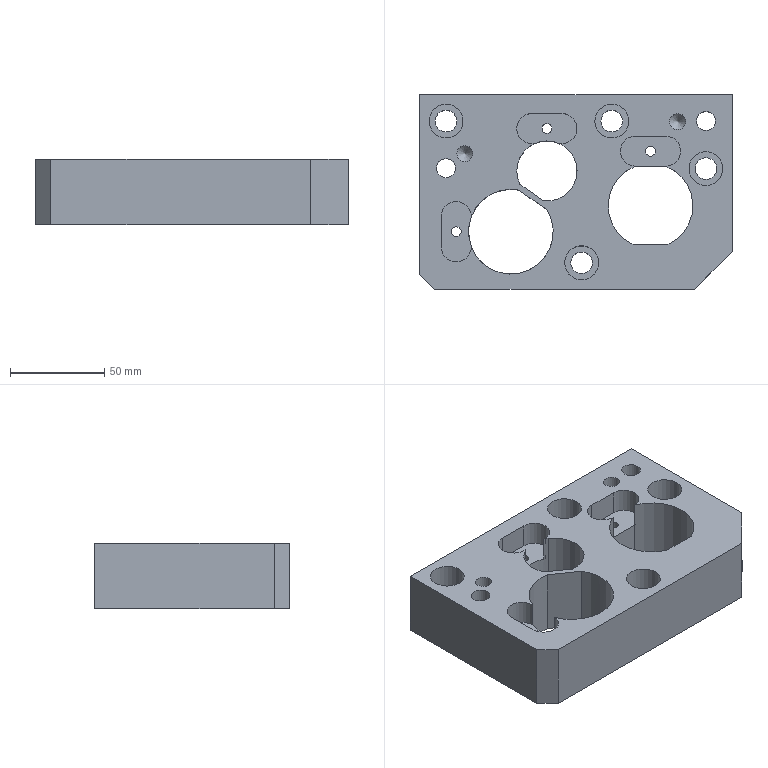Part | STEP file | lll_id4526_x_t | 1 solid | 52 faces | box 166 x 103.25 x 35 mm | volume 405165 mm3 | cylinder 26 | plane 24 | cone 2 | commonest cylinder face diameters 16 x6 11.509 x4 18.008 x4 5.206 x3 45 x3 8.506 x2
STEP:
#1=CARTESIAN_POINT('',(3428.774,36.5,-35.));
#2=VERTEX_POINT('',#1);
#3=CARTESIAN_POINT('',(3427.578,78.,-35.));
#4=VERTEX_POINT('',#3);
#5=CARTESIAN_POINT('',(3419.5,57.,-35.));
#6=DIRECTION('',(0.,0.,1.));
#7=DIRECTION('',(-1.,0.,0.));
#8=AXIS2_PLACEMENT_3D('',#5,#6,#7);
#9=CIRCLE('',#8,22.5);
#10=EDGE_CURVE('',#2,#4,#9,.T.);
#11=ORIENTED_EDGE('',*,*,#10,.F.);
#12=CARTESIAN_POINT('',(3428.774,36.5,0.));
#13=VERTEX_POINT('',#12);
#14=CARTESIAN_POINT('',(3428.774,36.5,0.));
#15=DIRECTION('',(0.,0.,-1.));
#16=VECTOR('',#15,1.);
#17=LINE('',#14,#16);
#18=EDGE_CURVE('',#13,#2,#17,.T.);
#19=ORIENTED_EDGE('',*,*,#18,.F.);
#20=CARTESIAN_POINT('',(3427.578,78.,0.));
#21=VERTEX_POINT('',#20);
#22=CARTESIAN_POINT('',(3419.5,57.,0.));
#23=DIRECTION('',(0.,0.,-1.));
#24=DIRECTION('',(1.,0.,0.));
#25=AXIS2_PLACEMENT_3D('',#22,#23,#24);
#26=CIRCLE('',#25,22.5);
#27=EDGE_CURVE('',#21,#13,#26,.T.);
#28=ORIENTED_EDGE('',*,*,#27,.F.);
#29=CARTESIAN_POINT('',(3427.578,78.,-30.));
#30=DIRECTION('',(0.,0.,-1.));
#31=VECTOR('',#30,1.);
#32=LINE('',#29,#31);
#33=EDGE_CURVE('',#21,#4,#32,.T.);
#34=ORIENTED_EDGE('',*,*,#33,.T.);
#35=EDGE_LOOP('',(#11,#19,#28,#34));
#36=FACE_OUTER_BOUND('',#35,.T.);
#37=CARTESIAN_POINT('',(3419.5,57.,-15.));
#38=DIRECTION('',(0.,0.,-1.));
#39=DIRECTION('',(0.,-1.,0.));
#40=AXIS2_PLACEMENT_3D('',#37,#38,#39);
#41=CYLINDRICAL_SURFACE('',#40,22.5);
#42=ADVANCED_FACE('',(#36),#41,.F.);
#43=CARTESIAN_POINT('',(3411.5,78.,0.));
#44=VERTEX_POINT('',#43);
#45=CARTESIAN_POINT('',(3411.5,78.,-13.));
#46=VERTEX_POINT('',#45);
#47=CARTESIAN_POINT('',(3411.5,78.,-6.5));
#48=DIRECTION('',(0.,0.,-1.));
#49=VECTOR('',#48,1.);
#50=LINE('',#47,#49);
#51=EDGE_CURVE('',#44,#46,#50,.T.);
#52=ORIENTED_EDGE('',*,*,#51,.F.);
#53=CARTESIAN_POINT('',(3411.422,78.,0.));
#54=VERTEX_POINT('',#53);
#55=CARTESIAN_POINT('',(3419.5,78.,0.));
#56=DIRECTION('',(-1.,0.,0.));
#57=VECTOR('',#56,1.);
#58=LINE('',#55,#57);
#59=EDGE_CURVE('',#44,#54,#58,.T.);
#60=ORIENTED_EDGE('',*,*,#59,.T.);
#61=CARTESIAN_POINT('',(3411.422,78.,-35.));
#62=VERTEX_POINT('',#61);
#63=CARTESIAN_POINT('',(3411.422,78.,0.00001771));
#64=DIRECTION('',(0.,0.,1.));
#65=VECTOR('',#64,1.);
#66=LINE('',#63,#65);
#67=EDGE_CURVE('',#62,#54,#66,.T.);
#68=ORIENTED_EDGE('',*,*,#67,.F.);
#69=CARTESIAN_POINT('',(3419.5,78.,-35.));
#70=DIRECTION('',(-1.,0.,0.));
#71=VECTOR('',#70,1.);
#72=LINE('',#69,#71);
#73=EDGE_CURVE('',#4,#62,#72,.T.);
#74=ORIENTED_EDGE('',*,*,#73,.F.);
#75=ORIENTED_EDGE('',*,*,#33,.F.);
#76=CARTESIAN_POINT('',(3427.5,78.,0.));
#77=VERTEX_POINT('',#76);
#78=CARTESIAN_POINT('',(3419.5,78.,0.));
#79=DIRECTION('',(-1.,0.,0.));
#80=VECTOR('',#79,1.);
#81=LINE('',#78,#80);
#82=EDGE_CURVE('',#21,#77,#81,.T.);
#83=ORIENTED_EDGE('',*,*,#82,.T.);
#84=CARTESIAN_POINT('',(3427.5,78.,-13.));
#85=VERTEX_POINT('',#84);
#86=CARTESIAN_POINT('',(3427.5,78.,-6.5));
#87=DIRECTION('',(0.,0.,-1.));
#88=VECTOR('',#87,1.);
#89=LINE('',#86,#88);
#90=EDGE_CURVE('',#77,#85,#89,.T.);
#91=ORIENTED_EDGE('',*,*,#90,.T.);
#92=CARTESIAN_POINT('',(3766.92,78.,-13.));
#93=DIRECTION('',(1.,0.,0.));
#94=VECTOR('',#93,1.);
#95=LINE('',#92,#94);
#96=EDGE_CURVE('',#46,#85,#95,.T.);
#97=ORIENTED_EDGE('',*,*,#96,.F.);
#98=EDGE_LOOP('',(#52,#60,#68,#74,#75,#83,#91,#97));
#99=FACE_OUTER_BOUND('',#98,.T.);
#100=CARTESIAN_POINT('',(3419.5,78.,-32.5));
#101=DIRECTION('',(0.,1.,0.));
#102=DIRECTION('',(0.,0.,-1.));
#103=AXIS2_PLACEMENT_3D('',#100,#101,#102);
#104=PLANE('',#103);
#105=ADVANCED_FACE('',(#99),#104,.F.);
#106=CARTESIAN_POINT('',(3357.736,90.,0.));
#107=VERTEX_POINT('',#106);
#108=CARTESIAN_POINT('',(3357.736,90.,-13.));
#109=VERTEX_POINT('',#108);
#110=CARTESIAN_POINT('',(3357.736,90.,-17.5));
#111=DIRECTION('',(0.,0.,-1.));
#112=VECTOR('',#111,1.);
#113=LINE('',#110,#112);
#114=EDGE_CURVE('',#107,#109,#113,.T.);
#115=ORIENTED_EDGE('',*,*,#114,.F.);
#116=CARTESIAN_POINT('',(3350.125,68.475,0.));
#117=VERTEX_POINT('',#116);
#118=CARTESIAN_POINT('',(3364.5,75.5,0.));
#119=DIRECTION('',(0.,0.,1.));
#120=DIRECTION('',(-1.,0.,0.));
#121=AXIS2_PLACEMENT_3D('',#118,#119,#120);
#122=CIRCLE('',#121,16.);
#123=EDGE_CURVE('',#107,#117,#122,.T.);
#124=ORIENTED_EDGE('',*,*,#123,.T.);
#125=CARTESIAN_POINT('',(3350.125,68.475,-35.));
#126=VERTEX_POINT('',#125);
#127=CARTESIAN_POINT('',(3350.125,68.475,-17.5));
#128=DIRECTION('',(0.,0.,-1.));
#129=VECTOR('',#128,1.);
#130=LINE('',#127,#129);
#131=EDGE_CURVE('',#117,#126,#130,.T.);
#132=ORIENTED_EDGE('',*,*,#131,.T.);
#133=CARTESIAN_POINT('',(3373.677,88.607,-35.));
#134=VERTEX_POINT('',#133);
#135=CARTESIAN_POINT('',(3364.5,75.5,-35.));
#136=DIRECTION('',(0.,0.,-1.));
#137=DIRECTION('',(-1.,0.,0.));
#138=AXIS2_PLACEMENT_3D('',#135,#136,#137);
#139=CIRCLE('',#138,16.);
#140=EDGE_CURVE('',#126,#134,#139,.T.);
#141=ORIENTED_EDGE('',*,*,#140,.T.);
#142=CARTESIAN_POINT('',(3373.677,88.607,0.));
#143=VERTEX_POINT('',#142);
#144=CARTESIAN_POINT('',(3373.677,88.607,-17.5));
#145=DIRECTION('',(0.,0.,-1.));
#146=VECTOR('',#145,1.);
#147=LINE('',#144,#146);
#148=EDGE_CURVE('',#143,#134,#147,.T.);
#149=ORIENTED_EDGE('',*,*,#148,.F.);
#150=CARTESIAN_POINT('',(3371.264,90.,0.));
#151=VERTEX_POINT('',#150);
#152=CARTESIAN_POINT('',(3364.5,75.5,0.));
#153=DIRECTION('',(0.,0.,1.));
#154=DIRECTION('',(-1.,0.,0.));
#155=AXIS2_PLACEMENT_3D('',#152,#153,#154);
#156=CIRCLE('',#155,16.);
#157=EDGE_CURVE('',#143,#151,#156,.T.);
#158=ORIENTED_EDGE('',*,*,#157,.T.);
#159=CARTESIAN_POINT('',(3371.264,90.,-13.));
#160=VERTEX_POINT('',#159);
#161=CARTESIAN_POINT('',(3371.264,90.,-17.5));
#162=DIRECTION('',(0.,0.,1.));
#163=VECTOR('',#162,1.);
#164=LINE('',#161,#163);
#165=EDGE_CURVE('',#160,#151,#164,.T.);
#166=ORIENTED_EDGE('',*,*,#165,.F.);
#167=CARTESIAN_POINT('',(3364.5,75.5,-13.));
#168=DIRECTION('',(0.,0.,-1.));
#169=DIRECTION('',(1.,0.,0.));
#170=AXIS2_PLACEMENT_3D('',#167,#168,#169);
#171=CIRCLE('',#170,16.);
#172=EDGE_CURVE('',#109,#160,#171,.T.);
#173=ORIENTED_EDGE('',*,*,#172,.F.);
#174=EDGE_LOOP('',(#115,#124,#132,#141,#149,#158,#166,#173));
#175=FACE_OUTER_BOUND('',#174,.T.);
#176=CARTESIAN_POINT('',(3364.5,75.5,-17.5));
#177=DIRECTION('',(0.,0.,1.));
#178=DIRECTION('',(-0.5736,-0.8192,0.));
#179=AXIS2_PLACEMENT_3D('',#176,#177,#178);
#180=CYLINDRICAL_SURFACE('',#179,16.);
#181=ADVANCED_FACE('',(#175),#180,.F.);
#182=ORIENTED_EDGE('',*,*,#27,.T.);
#183=CARTESIAN_POINT('',(3410.226,36.5,0.));
#184=VERTEX_POINT('',#183);
#185=CARTESIAN_POINT('',(0.,36.5,0.));
#186=DIRECTION('',(1.,0.,0.));
#187=VECTOR('',#186,1.);
#188=LINE('',#185,#187);
#189=EDGE_CURVE('',#184,#13,#188,.T.);
#190=ORIENTED_EDGE('',*,*,#189,.F.);
#191=CARTESIAN_POINT('',(3419.5,57.,0.));
#192=DIRECTION('',(0.,0.,-1.));
#193=DIRECTION('',(1.,0.,0.));
#194=AXIS2_PLACEMENT_3D('',#191,#192,#193);
#195=CIRCLE('',#194,22.5);
#196=EDGE_CURVE('',#184,#54,#195,.T.);
#197=ORIENTED_EDGE('',*,*,#196,.T.);
#198=ORIENTED_EDGE('',*,*,#59,.F.);
#199=CARTESIAN_POINT('',(3411.5,94.,0.));
#200=VERTEX_POINT('',#199);
#201=CARTESIAN_POINT('',(3411.5,86.,0.));
#202=DIRECTION('',(0.,0.,1.));
#203=DIRECTION('',(0.,-1.,0.));
#204=AXIS2_PLACEMENT_3D('',#201,#202,#203);
#205=CIRCLE('',#204,8.);
#206=EDGE_CURVE('',#200,#44,#205,.T.);
#207=ORIENTED_EDGE('',*,*,#206,.F.);
#208=CARTESIAN_POINT('',(3427.5,94.,0.));
#209=VERTEX_POINT('',#208);
#210=CARTESIAN_POINT('',(3408.538,94.,0.));
#211=DIRECTION('',(1.,0.,0.));
#212=VECTOR('',#211,1.);
#213=LINE('',#210,#212);
#214=EDGE_CURVE('',#200,#209,#213,.T.);
#215=ORIENTED_EDGE('',*,*,#214,.T.);
#216=CARTESIAN_POINT('',(3427.5,86.,0.));
#217=DIRECTION('',(0.,0.,1.));
#218=DIRECTION('',(0.,-1.,0.));
#219=AXIS2_PLACEMENT_3D('',#216,#217,#218);
#220=CIRCLE('',#219,8.);
#221=EDGE_CURVE('',#77,#209,#220,.T.);
#222=ORIENTED_EDGE('',*,*,#221,.F.);
#223=ORIENTED_EDGE('',*,*,#82,.F.);
#224=EDGE_LOOP('',(#182,#190,#197,#198,#207,#215,#222,#223));
#225=FACE_BOUND('',#224,.T.);
#226=CARTESIAN_POINT('',(3308.367,35.288,0.));
#227=VERTEX_POINT('',#226);
#228=CARTESIAN_POINT('',(3324.366,35.211,0.));
#229=VERTEX_POINT('',#228);
#230=CARTESIAN_POINT('',(3316.367,35.288,0.));
#231=DIRECTION('',(0.,0.,1.));
#232=DIRECTION('',(1.,0.,0.));
#233=AXIS2_PLACEMENT_3D('',#230,#231,#232);
#234=CIRCLE('',#233,8.);
#235=EDGE_CURVE('',#227,#229,#234,.T.);
#236=ORIENTED_EDGE('',*,*,#235,.F.);
#237=CARTESIAN_POINT('',(3308.367,51.288,0.));
#238=VERTEX_POINT('',#237);
#239=CARTESIAN_POINT('',(3308.367,32.325,0.));
#240=DIRECTION('',(0.,1.,0.));
#241=VECTOR('',#240,1.);
#242=LINE('',#239,#241);
#243=EDGE_CURVE('',#227,#238,#242,.T.);
#244=ORIENTED_EDGE('',*,*,#243,.T.);
#245=CARTESIAN_POINT('',(3324.366,51.364,0.));
#246=VERTEX_POINT('',#245);
#247=CARTESIAN_POINT('',(3316.367,51.288,0.));
#248=DIRECTION('',(0.,0.,1.));
#249=DIRECTION('',(1.,0.,0.));
#250=AXIS2_PLACEMENT_3D('',#247,#248,#249);
#251=CIRCLE('',#250,8.);
#252=EDGE_CURVE('',#246,#238,#251,.T.);
#253=ORIENTED_EDGE('',*,*,#252,.F.);
#254=CARTESIAN_POINT('',(3349.528,65.399,0.));
#255=VERTEX_POINT('',#254);
#256=CARTESIAN_POINT('',(3345.367,43.288,0.));
#257=DIRECTION('',(0.,0.,1.));
#258=DIRECTION('',(1.,0.,0.));
#259=AXIS2_PLACEMENT_3D('',#256,#257,#258);
#260=CIRCLE('',#259,22.5);
#261=EDGE_CURVE('',#255,#246,#260,.T.);
#262=ORIENTED_EDGE('',*,*,#261,.F.);
#263=CARTESIAN_POINT('',(3364.721,54.761,0.));
#264=VERTEX_POINT('',#263);
#265=CARTESIAN_POINT('',(3357.125,60.08,0.));
#266=DIRECTION('',(-0.8192,0.5736,0.));
#267=VECTOR('',#266,1.);
#268=LINE('',#265,#267);
#269=EDGE_CURVE('',#264,#255,#268,.T.);
#270=ORIENTED_EDGE('',*,*,#269,.F.);
#271=CARTESIAN_POINT('',(3345.367,43.288,0.));
#272=DIRECTION('',(0.,0.,1.));
#273=DIRECTION('',(1.,0.,0.));
#274=AXIS2_PLACEMENT_3D('',#271,#272,#273);
#275=CIRCLE('',#274,22.5);
#276=EDGE_CURVE('',#229,#264,#275,.T.);
#277=ORIENTED_EDGE('',*,*,#276,.F.);
#278=EDGE_LOOP('',(#236,#244,#253,#262,#270,#277));
#279=FACE_BOUND('',#278,.T.);
#280=CARTESIAN_POINT('',(3442.935,12.75,0.));
#281=VERTEX_POINT('',#280);
#282=CARTESIAN_POINT('',(3304.935,12.75,0.));
#283=VERTEX_POINT('',#282);
#284=CARTESIAN_POINT('',(3266.435,12.75,0.));
#285=DIRECTION('',(-1.,0.,0.));
#286=VECTOR('',#285,1.);
#287=LINE('',#284,#286);
#288=EDGE_CURVE('',#281,#283,#287,.T.);
#289=ORIENTED_EDGE('',*,*,#288,.F.);
#290=CARTESIAN_POINT('',(3462.935,32.75,0.));
#291=VERTEX_POINT('',#290);
#292=CARTESIAN_POINT('',(3455.935,25.75,0.));
#293=DIRECTION('',(0.7071,0.7071,0.));
#294=VECTOR('',#293,1.);
#295=LINE('',#292,#294);
#296=EDGE_CURVE('',#281,#291,#295,.T.);
#297=ORIENTED_EDGE('',*,*,#296,.T.);
#298=CARTESIAN_POINT('',(3462.935,116.,0.));
#299=VERTEX_POINT('',#298);
#300=CARTESIAN_POINT('',(3462.935,215.25,0.));
#301=DIRECTION('',(0.,-1.,0.));
#302=VECTOR('',#301,1.);
#303=LINE('',#300,#302);
#304=EDGE_CURVE('',#299,#291,#303,.T.);
#305=ORIENTED_EDGE('',*,*,#304,.F.);
#306=CARTESIAN_POINT('',(3296.935,116.,0.));
#307=VERTEX_POINT('',#306);
#308=CARTESIAN_POINT('',(3266.435,116.,0.));
#309=DIRECTION('',(-1.,0.,0.));
#310=VECTOR('',#309,1.);
#311=LINE('',#308,#310);
#312=EDGE_CURVE('',#299,#307,#311,.T.);
#313=ORIENTED_EDGE('',*,*,#312,.T.);
#314=CARTESIAN_POINT('',(3296.935,20.75,0.));
#315=VERTEX_POINT('',#314);
#316=CARTESIAN_POINT('',(3296.935,215.25,0.));
#317=DIRECTION('',(0.,-1.,0.));
#318=VECTOR('',#317,1.);
#319=LINE('',#316,#318);
#320=EDGE_CURVE('',#307,#315,#319,.T.);
#321=ORIENTED_EDGE('',*,*,#320,.T.);
#322=CARTESIAN_POINT('',(3179.435,138.25,0.));
#323=DIRECTION('',(0.7071,-0.7071,0.));
#324=VECTOR('',#323,1.);
#325=LINE('',#322,#324);
#326=EDGE_CURVE('',#315,#283,#325,.T.);
#327=ORIENTED_EDGE('',*,*,#326,.T.);
#328=EDGE_LOOP('',(#289,#297,#305,#313,#321,#327));
#329=FACE_BOUND('',#328,.T.);
#330=CARTESIAN_POINT('',(3319.939,102.,0.));
#331=VERTEX_POINT('',#330);
#332=CARTESIAN_POINT('',(3310.935,102.,0.));
#333=DIRECTION('',(0.,0.,1.));
#334=DIRECTION('',(1.,0.,0.));
#335=AXIS2_PLACEMENT_3D('',#332,#333,#334);
#336=CIRCLE('',#335,9.004);
#337=EDGE_CURVE('',#331,#331,#336,.T.);
#338=ORIENTED_EDGE('',*,*,#337,.F.);
#339=EDGE_LOOP('',(#338));
#340=FACE_BOUND('',#339,.T.);
#341=CARTESIAN_POINT('',(3315.935,77.,0.));
#342=VERTEX_POINT('',#341);
#343=CARTESIAN_POINT('',(3310.935,77.,0.));
#344=DIRECTION('',(0.,0.,1.));
#345=DIRECTION('',(1.,0.,0.));
#346=AXIS2_PLACEMENT_3D('',#343,#344,#345);
#347=CIRCLE('',#346,5.);
#348=EDGE_CURVE('',#342,#342,#347,.T.);
#349=ORIENTED_EDGE('',*,*,#348,.F.);
#350=EDGE_LOOP('',(#349));
#351=FACE_BOUND('',#350,.T.);
#352=CARTESIAN_POINT('',(3325.188,84.75,0.));
#353=VERTEX_POINT('',#352);
#354=CARTESIAN_POINT('',(3320.935,84.75,0.));
#355=DIRECTION('',(0.,0.,1.));
#356=DIRECTION('',(1.,0.,0.));
#357=AXIS2_PLACEMENT_3D('',#354,#355,#356);
#358=CIRCLE('',#357,4.253);
#359=EDGE_CURVE('',#353,#353,#358,.T.);
#360=ORIENTED_EDGE('',*,*,#359,.F.);
#361=EDGE_LOOP('',(#360));
#362=FACE_BOUND('',#361,.T.);
#363=CARTESIAN_POINT('',(3391.939,26.75,0.));
#364=VERTEX_POINT('',#363);
#365=CARTESIAN_POINT('',(3382.935,26.75,0.));
#366=DIRECTION('',(0.,0.,1.));
#367=DIRECTION('',(1.,0.,0.));
#368=AXIS2_PLACEMENT_3D('',#365,#366,#367);
#369=CIRCLE('',#368,9.004);
#370=EDGE_CURVE('',#364,#364,#369,.T.);
#371=ORIENTED_EDGE('',*,*,#370,.F.);
#372=EDGE_LOOP('',(#371));
#373=FACE_BOUND('',#372,.T.);
#374=CARTESIAN_POINT('',(3457.939,76.75,0.));
#375=VERTEX_POINT('',#374);
#376=CARTESIAN_POINT('',(3448.935,76.75,0.));
#377=DIRECTION('',(0.,0.,1.));
#378=DIRECTION('',(1.,0.,0.));
#379=AXIS2_PLACEMENT_3D('',#376,#377,#378);
#380=CIRCLE('',#379,9.004);
#381=EDGE_CURVE('',#375,#375,#380,.T.);
#382=ORIENTED_EDGE('',*,*,#381,.F.);
#383=EDGE_LOOP('',(#382));
#384=FACE_BOUND('',#383,.T.);
#385=CARTESIAN_POINT('',(3453.935,102.,0.));
#386=VERTEX_POINT('',#385);
#387=CARTESIAN_POINT('',(3448.935,102.,0.));
#388=DIRECTION('',(0.,0.,1.));
#389=DIRECTION('',(1.,0.,0.));
#390=AXIS2_PLACEMENT_3D('',#387,#388,#389);
#391=CIRCLE('',#390,5.);
#392=EDGE_CURVE('',#386,#386,#391,.T.);
#393=ORIENTED_EDGE('',*,*,#392,.F.);
#394=EDGE_LOOP('',(#393));
#395=FACE_BOUND('',#394,.T.);
#396=CARTESIAN_POINT('',(3407.939,102.,0.));
#397=VERTEX_POINT('',#396);
#398=CARTESIAN_POINT('',(3398.935,102.,0.));
#399=DIRECTION('',(0.,0.,1.));
#400=DIRECTION('',(1.,0.,0.));
#401=AXIS2_PLACEMENT_3D('',#398,#399,#400);
#402=CIRCLE('',#401,9.004);
#403=EDGE_CURVE('',#397,#397,#402,.T.);
#404=ORIENTED_EDGE('',*,*,#403,.F.);
#405=EDGE_LOOP('',(#404));
#406=FACE_BOUND('',#405,.T.);
#407=CARTESIAN_POINT('',(3438.188,101.75,0.));
#408=VERTEX_POINT('',#407);
#409=CARTESIAN_POINT('',(3433.935,101.75,0.));
#410=DIRECTION('',(0.,0.,1.));
#411=DIRECTION('',(1.,0.,0.));
#412=AXIS2_PLACEMENT_3D('',#409,#410,#411);
#413=CIRCLE('',#412,4.253);
#414=EDGE_CURVE('',#408,#408,#413,.T.);
#415=ORIENTED_EDGE('',*,*,#414,.F.);
#416=EDGE_LOOP('',(#415));
#417=FACE_BOUND('',#416,.T.);
#418=ORIENTED_EDGE('',*,*,#123,.F.);
#419=CARTESIAN_POINT('',(3356.5,90.,0.));
#420=VERTEX_POINT('',#419);
#421=CARTESIAN_POINT('',(3353.538,90.,0.));
#422=DIRECTION('',(-1.,0.,0.));
#423=VECTOR('',#422,1.);
#424=LINE('',#421,#423);
#425=EDGE_CURVE('',#107,#420,#424,.T.);
#426=ORIENTED_EDGE('',*,*,#425,.T.);
#427=CARTESIAN_POINT('',(3356.5,106.,0.));
#428=VERTEX_POINT('',#427);
#429=CARTESIAN_POINT('',(3356.5,98.,0.));
#430=DIRECTION('',(0.,0.,1.));
#431=DIRECTION('',(0.,-1.,0.));
#432=AXIS2_PLACEMENT_3D('',#429,#430,#431);
#433=CIRCLE('',#432,8.);
#434=EDGE_CURVE('',#428,#420,#433,.T.);
#435=ORIENTED_EDGE('',*,*,#434,.F.);
#436=CARTESIAN_POINT('',(3372.5,106.,0.));
#437=VERTEX_POINT('',#436);
#438=CARTESIAN_POINT('',(3353.538,106.,0.));
#439=DIRECTION('',(1.,0.,0.));
#440=VECTOR('',#439,1.);
#441=LINE('',#438,#440);
#442=EDGE_CURVE('',#428,#437,#441,.T.);
#443=ORIENTED_EDGE('',*,*,#442,.T.);
#444=CARTESIAN_POINT('',(3372.5,90.,0.));
#445=VERTEX_POINT('',#444);
#446=CARTESIAN_POINT('',(3372.5,98.,0.));
#447=DIRECTION('',(0.,0.,1.));
#448=DIRECTION('',(0.,-1.,0.));
#449=AXIS2_PLACEMENT_3D('',#446,#447,#448);
#450=CIRCLE('',#449,8.);
#451=EDGE_CURVE('',#445,#437,#450,.T.);
#452=ORIENTED_EDGE('',*,*,#451,.F.);
#453=CARTESIAN_POINT('',(3353.538,90.,0.));
#454=DIRECTION('',(-1.,0.,0.));
#455=VECTOR('',#454,1.);
#456=LINE('',#453,#455);
#457=EDGE_CURVE('',#445,#151,#456,.T.);
#458=ORIENTED_EDGE('',*,*,#457,.T.);
#459=ORIENTED_EDGE('',*,*,#157,.F.);
#460=CARTESIAN_POINT('',(3362.815,59.589,0.000008705));
#461=VERTEX_POINT('',#460);
#462=CARTESIAN_POINT('',(3364.5,75.5,0.));
#463=DIRECTION('',(0.,0.,1.));
#464=DIRECTION('',(-1.,0.,0.));
#465=AXIS2_PLACEMENT_3D('',#462,#463,#464);
#466=CIRCLE('',#465,16.);
#467=EDGE_CURVE('',#461,#143,#466,.T.);
#468=ORIENTED_EDGE('',*,*,#467,.F.);
#469=CARTESIAN_POINT('',(3225.007,156.084,0.));
#470=DIRECTION('',(0.8192,-0.5736,0.));
#471=VECTOR('',#470,1.);
#472=LINE('',#469,#471);
#473=EDGE_CURVE('',#117,#461,#472,.T.);
#474=ORIENTED_EDGE('',*,*,#473,.F.);
#475=EDGE_LOOP('',(#418,#426,#435,#443,#452,#458,#459,#468,#474));
#476=FACE_BOUND('',#475,.T.);
#477=CARTESIAN_POINT('',(3266.435,215.25,0.));
#478=DIRECTION('',(0.,0.,1.));
#479=DIRECTION('',(-1.,0.,0.));
#480=AXIS2_PLACEMENT_3D('',#477,#478,#479);
#481=PLANE('',#480);
#482=ADVANCED_FACE('',(#225,#279,#329,#340,#351,#362,#373,#384,#395,#406,#417,#476),#481,.T.);
#483=CARTESIAN_POINT('',(3324.366,35.211,-13.));
#484=VERTEX_POINT('',#483);
#485=CARTESIAN_POINT('',(3324.366,51.364,-13.));
#486=VERTEX_POINT('',#485);
#487=CARTESIAN_POINT('',(3345.367,43.288,-13.));
#488=DIRECTION('',(0.,0.,-1.));
#489=DIRECTION('',(1.,0.,0.));
#490=AXIS2_PLACEMENT_3D('',#487,#488,#489);
#491=CIRCLE('',#490,22.5);
#492=EDGE_CURVE('',#484,#486,#491,.T.);
#493=ORIENTED_EDGE('',*,*,#492,.F.);
#494=CARTESIAN_POINT('',(3324.366,35.211,-6.5));
#495=DIRECTION('',(0.,0.,1.));
#496=VECTOR('',#495,1.);
#497=LINE('',#494,#496);
#498=EDGE_CURVE('',#484,#229,#497,.T.);
#499=ORIENTED_EDGE('',*,*,#498,.T.);
#500=ORIENTED_EDGE('',*,*,#276,.T.);
#501=CARTESIAN_POINT('',(3364.721,54.761,-35.));
#502=VERTEX_POINT('',#501);
#503=CARTESIAN_POINT('',(3364.721,54.761,-15.));
#504=DIRECTION('',(0.,0.,-1.));
#505=VECTOR('',#504,1.);
#506=LINE('',#503,#505);
#507=EDGE_CURVE('',#264,#502,#506,.T.);
#508=ORIENTED_EDGE('',*,*,#507,.T.);
#509=CARTESIAN_POINT('',(3349.528,65.399,-35.));
#510=VERTEX_POINT('',#509);
#511=CARTESIAN_POINT('',(3345.367,43.288,-35.));
#512=DIRECTION('',(0.,0.,1.));
#513=DIRECTION('',(-1.,0.,0.));
#514=AXIS2_PLACEMENT_3D('',#511,#512,#513);
#515=CIRCLE('',#514,22.5);
#516=EDGE_CURVE('',#510,#502,#515,.T.);
#517=ORIENTED_EDGE('',*,*,#516,.F.);
#518=CARTESIAN_POINT('',(3349.528,65.399,-15.));
#519=DIRECTION('',(0.,0.,1.));
#520=VECTOR('',#519,1.);
#521=LINE('',#518,#520);
#522=EDGE_CURVE('',#510,#255,#521,.T.);
#523=ORIENTED_EDGE('',*,*,#522,.T.);
#524=ORIENTED_EDGE('',*,*,#261,.T.);
#525=CARTESIAN_POINT('',(3324.366,51.364,-6.5));
#526=DIRECTION('',(0.,0.,-1.));
#527=VECTOR('',#526,1.);
#528=LINE('',#525,#527);
#529=EDGE_CURVE('',#246,#486,#528,.T.);
#530=ORIENTED_EDGE('',*,*,#529,.T.);
#531=EDGE_LOOP('',(#493,#499,#500,#508,#517,#523,#524,#530));
#532=FACE_OUTER_BOUND('',#531,.T.);
#533=CARTESIAN_POINT('',(3345.367,43.288,-15.));
#534=DIRECTION('',(0.,0.,-1.));
#535=DIRECTION('',(0.8192,-0.5736,0.));
#536=AXIS2_PLACEMENT_3D('',#533,#534,#535);
#537=CYLINDRICAL_SURFACE('',#536,22.5);
#538=ADVANCED_FACE('',(#532),#537,.F.);
#539=ORIENTED_EDGE('',*,*,#467,.T.);
#540=ORIENTED_EDGE('',*,*,#148,.T.);
#541=CARTESIAN_POINT('',(3362.815,59.589,-35.));
#542=VERTEX_POINT('',#541);
#543=CARTESIAN_POINT('',(3364.5,75.5,-35.));
#544=DIRECTION('',(0.,0.,-1.));
#545=DIRECTION('',(-1.,0.,0.));
#546=AXIS2_PLACEMENT_3D('',#543,#544,#545);
#547=CIRCLE('',#546,16.);
#548=EDGE_CURVE('',#134,#542,#547,.T.);
#549=ORIENTED_EDGE('',*,*,#548,.T.);
#550=CARTESIAN_POINT('',(3362.815,59.589,-17.5));
#551=DIRECTION('',(0.,0.,1.));
#552=VECTOR('',#551,1.);
#553=LINE('',#550,#552);
#554=EDGE_CURVE('',#542,#461,#553,.T.);
#555=ORIENTED_EDGE('',*,*,#554,.T.);
#556=EDGE_LOOP('',(#539,#540,#549,#555));
#557=FACE_OUTER_BOUND('',#556,.T.);
#558=CARTESIAN_POINT('',(3364.5,75.5,-17.5));
#559=DIRECTION('',(0.,0.,1.));
#560=DIRECTION('',(-0.5736,-0.8192,0.));
#561=AXIS2_PLACEMENT_3D('',#558,#559,#560);
#562=CYLINDRICAL_SURFACE('',#561,16.);
#563=ADVANCED_FACE('',(#557),#562,.F.);
#564=CARTESIAN_POINT('',(3410.226,36.5,-35.));
#565=VERTEX_POINT('',#564);
#566=CARTESIAN_POINT('',(3410.226,36.5,-15.));
#567=DIRECTION('',(0.,0.,1.));
#568=VECTOR('',#567,1.);
#569=LINE('',#566,#568);
#570=EDGE_CURVE('',#565,#184,#569,.T.);
#571=ORIENTED_EDGE('',*,*,#570,.F.);
#572=CARTESIAN_POINT('',(3419.5,57.,-35.));
#573=DIRECTION('',(0.,0.,1.));
#574=DIRECTION('',(-1.,0.,0.));
#575=AXIS2_PLACEMENT_3D('',#572,#573,#574);
#576=CIRCLE('',#575,22.5);
#577=EDGE_CURVE('',#62,#565,#576,.T.);
#578=ORIENTED_EDGE('',*,*,#577,.F.);
#579=ORIENTED_EDGE('',*,*,#67,.T.);
#580=ORIENTED_EDGE('',*,*,#196,.F.);
#581=EDGE_LOOP('',(#571,#578,#579,#580));
#582=FACE_OUTER_BOUND('',#581,.T.);
#583=CARTESIAN_POINT('',(3419.5,57.,-15.));
#584=DIRECTION('',(0.,0.,-1.));
#585=DIRECTION('',(0.,-1.,0.));
#586=AXIS2_PLACEMENT_3D('',#583,#584,#585);
#587=CYLINDRICAL_SURFACE('',#586,22.5);
#588=ADVANCED_FACE('',(#582),#587,.F.);
#589=ORIENTED_EDGE('',*,*,#522,.F.);
#590=CARTESIAN_POINT('',(3357.125,60.08,-35.));
#591=DIRECTION('',(0.8192,-0.5736,0.));
#592=VECTOR('',#591,1.);
#593=LINE('',#590,#592);
#594=EDGE_CURVE('',#510,#502,#593,.T.);
#595=ORIENTED_EDGE('',*,*,#594,.T.);
#596=ORIENTED_EDGE('',*,*,#507,.F.);
#597=ORIENTED_EDGE('',*,*,#269,.T.);
#598=EDGE_LOOP('',(#589,#595,#596,#597));
#599=FACE_OUTER_BOUND('',#598,.T.);
#600=CARTESIAN_POINT('',(3357.125,60.08,-32.5));
#601=DIRECTION('',(0.5736,0.8192,0.));
#602=DIRECTION('',(0.,0.,1.));
#603=AXIS2_PLACEMENT_3D('',#600,#601,#602);
#604=PLANE('',#603);
#605=ADVANCED_FACE('',(#599),#604,.F.);
#606=ORIENTED_EDGE('',*,*,#554,.F.);
#607=CARTESIAN_POINT('',(3225.007,156.084,-35.));
#608=DIRECTION('',(-0.8192,0.5736,0.));
#609=VECTOR('',#608,1.);
#610=LINE('',#607,#609);
#611=EDGE_CURVE('',#542,#126,#610,.T.);
#612=ORIENTED_EDGE('',*,*,#611,.T.);
#613=ORIENTED_EDGE('',*,*,#131,.F.);
#614=ORIENTED_EDGE('',*,*,#473,.T.);
#615=EDGE_LOOP('',(#606,#612,#613,#614));
#616=FACE_OUTER_BOUND('',#615,.T.);
#617=CARTESIAN_POINT('',(3356.47,64.032,-32.5));
#618=DIRECTION('',(-0.5736,-0.8192,0.));
#619=DIRECTION('',(0.,0.,-1.));
#620=AXIS2_PLACEMENT_3D('',#617,#618,#619);
#621=PLANE('',#620);
#622=ADVANCED_FACE('',(#616),#621,.F.);
#623=CARTESIAN_POINT('',(3304.935,12.75,-35.));
#624=VERTEX_POINT('',#623);
#625=CARTESIAN_POINT('',(3442.935,12.75,-35.));
#626=VERTEX_POINT('',#625);
#627=CARTESIAN_POINT('',(3266.435,12.75,-35.));
#628=DIRECTION('',(1.,0.,0.));
#629=VECTOR('',#628,1.);
#630=LINE('',#627,#629);
#631=EDGE_CURVE('',#624,#626,#630,.T.);
#632=ORIENTED_EDGE('',*,*,#631,.T.);
#633=CARTESIAN_POINT('',(3442.935,12.75,-32.));
#634=DIRECTION('',(0.,0.,1.));
#635=VECTOR('',#634,1.);
#636=LINE('',#633,#635);
#637=EDGE_CURVE('',#626,#281,#636,.T.);
#638=ORIENTED_EDGE('',*,*,#637,.T.);
#639=ORIENTED_EDGE('',*,*,#288,.T.);
#640=CARTESIAN_POINT('',(3304.935,12.75,-35.));
#641=DIRECTION('',(0.,0.,-1.));
#642=VECTOR('',#641,1.);
#643=LINE('',#640,#642);
#644=EDGE_CURVE('',#283,#624,#643,.T.);
#645=ORIENTED_EDGE('',*,*,#644,.T.);
#646=EDGE_LOOP('',(#632,#638,#639,#645));
#647=FACE_OUTER_BOUND('',#646,.T.);
#648=CARTESIAN_POINT('',(3266.435,12.75,-32.));
#649=DIRECTION('',(0.,-1.,0.));
#650=DIRECTION('',(0.,0.,1.));
#651=AXIS2_PLACEMENT_3D('',#648,#649,#650);
#652=PLANE('',#651);
#653=ADVANCED_FACE('',(#647),#652,.T.);
#654=ORIENTED_EDGE('',*,*,#304,.T.);
#655=CARTESIAN_POINT('',(3462.935,32.75,-35.));
#656=VERTEX_POINT('',#655);
#657=CARTESIAN_POINT('',(3462.935,32.75,-32.));
#658=DIRECTION('',(0.,0.,-1.));
#659=VECTOR('',#658,1.);
#660=LINE('',#657,#659);
#661=EDGE_CURVE('',#291,#656,#660,.T.);
#662=ORIENTED_EDGE('',*,*,#661,.T.);
#663=CARTESIAN_POINT('',(3462.935,116.,-35.));
#664=VERTEX_POINT('',#663);
#665=CARTESIAN_POINT('',(3462.935,215.25,-35.));
#666=DIRECTION('',(0.,1.,0.));
#667=VECTOR('',#666,1.);
#668=LINE('',#665,#667);
#669=EDGE_CURVE('',#656,#664,#668,.T.);
#670=ORIENTED_EDGE('',*,*,#669,.T.);
#671=CARTESIAN_POINT('',(3462.935,116.,-32.));
#672=DIRECTION('',(0.,0.,1.));
#673=VECTOR('',#672,1.);
#674=LINE('',#671,#673);
#675=EDGE_CURVE('',#664,#299,#674,.T.);
#676=ORIENTED_EDGE('',*,*,#675,.T.);
#677=EDGE_LOOP('',(#654,#662,#670,#676));
#678=FACE_OUTER_BOUND('',#677,.T.);
#679=CARTESIAN_POINT('',(3462.935,215.25,-32.));
#680=DIRECTION('',(1.,0.,0.));
#681=DIRECTION('',(0.,0.,1.));
#682=AXIS2_PLACEMENT_3D('',#679,#680,#681);
#683=PLANE('',#682);
#684=ADVANCED_FACE('',(#678),#683,.T.);
#685=CARTESIAN_POINT('',(3313.764,43.288,-35.));
#686=VERTEX_POINT('',#685);
#687=CARTESIAN_POINT('',(3316.367,43.288,-35.));
#688=DIRECTION('',(0.,0.,-1.));
#689=DIRECTION('',(-1.,0.,0.));
#690=AXIS2_PLACEMENT_3D('',#687,#688,#689);
#691=CIRCLE('',#690,2.603);
#692=EDGE_CURVE('',#686,#686,#691,.T.);
#693=ORIENTED_EDGE('',*,*,#692,.F.);
#694=EDGE_LOOP('',(#693));
#695=FACE_BOUND('',#694,.T.);
#696=CARTESIAN_POINT('',(3419.5,88.603,-35.));
#697=VERTEX_POINT('',#696);
#698=CARTESIAN_POINT('',(3419.5,86.,-35.));
#699=DIRECTION('',(0.,0.,-1.));
#700=DIRECTION('',(0.,1.,0.));
#701=AXIS2_PLACEMENT_3D('',#698,#699,#700);
#702=CIRCLE('',#701,2.603);
#703=EDGE_CURVE('',#697,#697,#702,.T.);
#704=ORIENTED_EDGE('',*,*,#703,.F.);
#705=EDGE_LOOP('',(#704));
#706=FACE_BOUND('',#705,.T.);
#707=CARTESIAN_POINT('',(3364.5,100.603,-35.));
#708=VERTEX_POINT('',#707);
#709=CARTESIAN_POINT('',(3364.5,98.,-35.));
#710=DIRECTION('',(0.,0.,-1.));
#711=DIRECTION('',(0.,1.,0.));
#712=AXIS2_PLACEMENT_3D('',#709,#710,#711);
#713=CIRCLE('',#712,2.603);
#714=EDGE_CURVE('',#708,#708,#713,.T.);
#715=ORIENTED_EDGE('',*,*,#714,.F.);
#716=EDGE_LOOP('',(#715));
#717=FACE_BOUND('',#716,.T.);
#718=ORIENTED_EDGE('',*,*,#516,.T.);
#719=ORIENTED_EDGE('',*,*,#594,.F.);
#720=EDGE_LOOP('',(#718,#719));
#721=FACE_BOUND('',#720,.T.);
#722=ORIENTED_EDGE('',*,*,#10,.T.);
#723=ORIENTED_EDGE('',*,*,#73,.T.);
#724=ORIENTED_EDGE('',*,*,#577,.T.);
#725=CARTESIAN_POINT('',(0.,36.5,-35.));
#726=DIRECTION('',(-1.,0.,0.));
#727=VECTOR('',#726,1.);
#728=LINE('',#725,#727);
#729=EDGE_CURVE('',#2,#565,#728,.T.);
#730=ORIENTED_EDGE('',*,*,#729,.F.);
#731=EDGE_LOOP('',(#722,#723,#724,#730));
#732=FACE_BOUND('',#731,.T.);
#733=ORIENTED_EDGE('',*,*,#611,.F.);
#734=ORIENTED_EDGE('',*,*,#548,.F.);
#735=ORIENTED_EDGE('',*,*,#140,.F.);
#736=EDGE_LOOP('',(#733,#734,#735));
#737=FACE_BOUND('',#736,.T.);
#738=CARTESIAN_POINT('',(3443.181,76.75,-35.));
#739=VERTEX_POINT('',#738);
#740=CARTESIAN_POINT('',(3448.935,76.75,-35.));
#741=DIRECTION('',(0.,0.,-1.));
#742=DIRECTION('',(-1.,0.,0.));
#743=AXIS2_PLACEMENT_3D('',#740,#741,#742);
#744=CIRCLE('',#743,5.755);
#745=EDGE_CURVE('',#739,#739,#744,.T.);
#746=ORIENTED_EDGE('',*,*,#745,.F.);
#747=EDGE_LOOP('',(#746));
#748=FACE_BOUND('',#747,.T.);
#749=CARTESIAN_POINT('',(3393.181,102.,-35.));
#750=VERTEX_POINT('',#749);
#751=CARTESIAN_POINT('',(3398.935,102.,-35.));
#752=DIRECTION('',(0.,0.,-1.));
#753=DIRECTION('',(-1.,0.,0.));
#754=AXIS2_PLACEMENT_3D('',#751,#752,#753);
#755=CIRCLE('',#754,5.755);
#756=EDGE_CURVE('',#750,#750,#755,.T.);
#757=ORIENTED_EDGE('',*,*,#756,.F.);
#758=EDGE_LOOP('',(#757));
#759=FACE_BOUND('',#758,.T.);
#760=CARTESIAN_POINT('',(3443.935,102.,-35.));
#761=VERTEX_POINT('',#760);
#762=CARTESIAN_POINT('',(3448.935,102.,-35.));
#763=DIRECTION('',(0.,0.,-1.));
#764=DIRECTION('',(-1.,0.,0.));
#765=AXIS2_PLACEMENT_3D('',#762,#763,#764);
#766=CIRCLE('',#765,5.);
#767=EDGE_CURVE('',#761,#761,#766,.T.);
#768=ORIENTED_EDGE('',*,*,#767,.F.);
#769=EDGE_LOOP('',(#768));
#770=FACE_BOUND('',#769,.T.);
#771=CARTESIAN_POINT('',(3377.181,26.75,-35.));
#772=VERTEX_POINT('',#771);
#773=CARTESIAN_POINT('',(3382.935,26.75,-35.));
#774=DIRECTION('',(0.,0.,-1.));
#775=DIRECTION('',(-1.,0.,0.));
#776=AXIS2_PLACEMENT_3D('',#773,#774,#775);
#777=CIRCLE('',#776,5.755);
#778=EDGE_CURVE('',#772,#772,#777,.T.);
#779=ORIENTED_EDGE('',*,*,#778,.F.);
#780=EDGE_LOOP('',(#779));
#781=FACE_BOUND('',#780,.T.);
#782=CARTESIAN_POINT('',(3305.935,77.,-35.));
#783=VERTEX_POINT('',#782);
#784=CARTESIAN_POINT('',(3310.935,77.,-35.));
#785=DIRECTION('',(0.,0.,-1.));
#786=DIRECTION('',(-1.,0.,0.));
#787=AXIS2_PLACEMENT_3D('',#784,#785,#786);
#788=CIRCLE('',#787,5.);
#789=EDGE_CURVE('',#783,#783,#788,.T.);
#790=ORIENTED_EDGE('',*,*,#789,.F.);
#791=EDGE_LOOP('',(#790));
#792=FACE_BOUND('',#791,.T.);
#793=CARTESIAN_POINT('',(3305.181,102.,-35.));
#794=VERTEX_POINT('',#793);
#795=CARTESIAN_POINT('',(3310.935,102.,-35.));
#796=DIRECTION('',(0.,0.,-1.));
#797=DIRECTION('',(-1.,0.,0.));
#798=AXIS2_PLACEMENT_3D('',#795,#796,#797);
#799=CIRCLE('',#798,5.755);
#800=EDGE_CURVE('',#794,#794,#799,.T.);
#801=ORIENTED_EDGE('',*,*,#800,.F.);
#802=EDGE_LOOP('',(#801));
#803=FACE_BOUND('',#802,.T.);
#804=ORIENTED_EDGE('',*,*,#669,.F.);
#805=CARTESIAN_POINT('',(3455.935,25.75,-35.));
#806=DIRECTION('',(-0.7071,-0.7071,0.));
#807=VECTOR('',#806,1.);
#808=LINE('',#805,#807);
#809=EDGE_CURVE('',#656,#626,#808,.T.);
#810=ORIENTED_EDGE('',*,*,#809,.T.);
#811=ORIENTED_EDGE('',*,*,#631,.F.);
#812=CARTESIAN_POINT('',(3296.935,20.75,-35.));
#813=VERTEX_POINT('',#812);
#814=CARTESIAN_POINT('',(3179.435,138.25,-35.));
#815=DIRECTION('',(-0.7071,0.7071,0.));
#816=VECTOR('',#815,1.);
#817=LINE('',#814,#816);
#818=EDGE_CURVE('',#624,#813,#817,.T.);
#819=ORIENTED_EDGE('',*,*,#818,.T.);
#820=CARTESIAN_POINT('',(3296.935,116.,-35.));
#821=VERTEX_POINT('',#820);
#822=CARTESIAN_POINT('',(3296.935,215.25,-35.));
#823=DIRECTION('',(0.,-1.,0.));
#824=VECTOR('',#823,1.);
#825=LINE('',#822,#824);
#826=EDGE_CURVE('',#821,#813,#825,.T.);
#827=ORIENTED_EDGE('',*,*,#826,.F.);
#828=CARTESIAN_POINT('',(3266.435,116.,-35.));
#829=DIRECTION('',(-1.,0.,0.));
#830=VECTOR('',#829,1.);
#831=LINE('',#828,#830);
#832=EDGE_CURVE('',#664,#821,#831,.T.);
#833=ORIENTED_EDGE('',*,*,#832,.F.);
#834=EDGE_LOOP('',(#804,#810,#811,#819,#827,#833));
#835=FACE_BOUND('',#834,.T.);
#836=CARTESIAN_POINT('',(3266.435,215.25,-35.));
#837=DIRECTION('',(0.,0.,-1.));
#838=DIRECTION('',(1.,0.,0.));
#839=AXIS2_PLACEMENT_3D('',#836,#837,#838);
#840=PLANE('',#839);
#841=ADVANCED_FACE('',(#695,#706,#717,#721,#732,#737,#748,#759,#770,#781,#792,#803,#835),#840,.T.);
#842=ORIENTED_EDGE('',*,*,#832,.T.);
#843=CARTESIAN_POINT('',(3296.935,116.,-17.5));
#844=DIRECTION('',(0.,0.,-1.));
#845=VECTOR('',#844,1.);
#846=LINE('',#843,#845);
#847=EDGE_CURVE('',#307,#821,#846,.T.);
#848=ORIENTED_EDGE('',*,*,#847,.F.);
#849=ORIENTED_EDGE('',*,*,#312,.F.);
#850=ORIENTED_EDGE('',*,*,#675,.F.);
#851=EDGE_LOOP('',(#842,#848,#849,#850));
#852=FACE_OUTER_BOUND('',#851,.T.);
#853=CARTESIAN_POINT('',(3384.935,116.,-17.5));
#854=DIRECTION('',(0.,-1.,0.));
#855=DIRECTION('',(0.,0.,-1.));
#856=AXIS2_PLACEMENT_3D('',#853,#854,#855);
#857=PLANE('',#856);
#858=ADVANCED_FACE('',(#852),#857,.F.);
#859=ORIENTED_EDGE('',*,*,#826,.T.);
#860=CARTESIAN_POINT('',(3296.935,20.75,0.));
#861=DIRECTION('',(0.,0.,1.));
#862=VECTOR('',#861,1.);
#863=LINE('',#860,#862);
#864=EDGE_CURVE('',#813,#315,#863,.T.);
#865=ORIENTED_EDGE('',*,*,#864,.T.);
#866=ORIENTED_EDGE('',*,*,#320,.F.);
#867=ORIENTED_EDGE('',*,*,#847,.T.);
#868=EDGE_LOOP('',(#859,#865,#866,#867));
#869=FACE_OUTER_BOUND('',#868,.T.);
#870=CARTESIAN_POINT('',(3296.935,62.,-17.5));
#871=DIRECTION('',(1.,0.,0.));
#872=DIRECTION('',(0.,0.,-1.));
#873=AXIS2_PLACEMENT_3D('',#870,#871,#872);
#874=PLANE('',#873);
#875=ADVANCED_FACE('',(#869),#874,.F.);
#876=ORIENTED_EDGE('',*,*,#800,.T.);
#877=EDGE_LOOP('',(#876));
#878=FACE_BOUND('',#877,.T.);
#879=CARTESIAN_POINT('',(3305.181,102.,-13.));
#880=VERTEX_POINT('',#879);
#881=CARTESIAN_POINT('',(3310.935,102.,-13.));
#882=DIRECTION('',(0.,0.,-1.));
#883=DIRECTION('',(-1.,0.,0.));
#884=AXIS2_PLACEMENT_3D('',#881,#882,#883);
#885=CIRCLE('',#884,5.755);
#886=EDGE_CURVE('',#880,#880,#885,.T.);
#887=ORIENTED_EDGE('',*,*,#886,.F.);
#888=EDGE_LOOP('',(#887));
#889=FACE_BOUND('',#888,.T.);
#890=CARTESIAN_POINT('',(3310.935,102.,2.));
#891=DIRECTION('',(0.,0.,-1.));
#892=DIRECTION('',(1.,0.,0.));
#893=AXIS2_PLACEMENT_3D('',#890,#891,#892);
#894=CYLINDRICAL_SURFACE('',#893,5.755);
#895=ADVANCED_FACE('',(#878,#889),#894,.F.);
#896=ORIENTED_EDGE('',*,*,#886,.T.);
#897=EDGE_LOOP('',(#896));
#898=FACE_BOUND('',#897,.T.);
#899=CARTESIAN_POINT('',(3319.939,102.,-13.));
#900=VERTEX_POINT('',#899);
#901=CARTESIAN_POINT('',(3310.935,102.,-13.));
#902=DIRECTION('',(0.,0.,-1.));
#903=DIRECTION('',(1.,0.,0.));
#904=AXIS2_PLACEMENT_3D('',#901,#902,#903);
#905=CIRCLE('',#904,9.004);
#906=EDGE_CURVE('',#900,#900,#905,.T.);
#907=ORIENTED_EDGE('',*,*,#906,.F.);
#908=EDGE_LOOP('',(#907));
#909=FACE_BOUND('',#908,.T.);
#910=CARTESIAN_POINT('',(3310.935,102.,-13.));
#911=DIRECTION('',(0.,0.,-1.));
#912=DIRECTION('',(-1.,0.,0.));
#913=AXIS2_PLACEMENT_3D('',#910,#911,#912);
#914=PLANE('',#913);
#915=ADVANCED_FACE('',(#898,#909),#914,.F.);
#916=ORIENTED_EDGE('',*,*,#337,.T.);
#917=EDGE_LOOP('',(#916));
#918=FACE_BOUND('',#917,.T.);
#919=ORIENTED_EDGE('',*,*,#906,.T.);
#920=EDGE_LOOP('',(#919));
#921=FACE_BOUND('',#920,.T.);
#922=CARTESIAN_POINT('',(3310.935,102.,0.00007723));
#923=DIRECTION('',(0.,0.,-1.));
#924=DIRECTION('',(1.,0.,0.));
#925=AXIS2_PLACEMENT_3D('',#922,#923,#924);
#926=CYLINDRICAL_SURFACE('',#925,9.004);
#927=ADVANCED_FACE('',(#918,#921),#926,.F.);
#928=ORIENTED_EDGE('',*,*,#789,.T.);
#929=EDGE_LOOP('',(#928));
#930=FACE_BOUND('',#929,.T.);
#931=ORIENTED_EDGE('',*,*,#348,.T.);
#932=EDGE_LOOP('',(#931));
#933=FACE_BOUND('',#932,.T.);
#934=CARTESIAN_POINT('',(3310.935,77.,2.));
#935=DIRECTION('',(0.,0.,-1.));
#936=DIRECTION('',(-1.,0.,0.));
#937=AXIS2_PLACEMENT_3D('',#934,#935,#936);
#938=CYLINDRICAL_SURFACE('',#937,5.);
#939=ADVANCED_FACE('',(#930,#933),#938,.F.);
#940=ORIENTED_EDGE('',*,*,#359,.T.);
#941=EDGE_LOOP('',(#940));
#942=FACE_BOUND('',#941,.T.);
#943=CARTESIAN_POINT('',(3325.188,84.75,-28.753));
#944=VERTEX_POINT('',#943);
#945=CARTESIAN_POINT('',(3320.935,84.75,-28.753));
#946=DIRECTION('',(0.,0.,1.));
#947=DIRECTION('',(1.,0.,0.));
#948=AXIS2_PLACEMENT_3D('',#945,#946,#947);
#949=CIRCLE('',#948,4.253);
#950=EDGE_CURVE('',#944,#944,#949,.T.);
#951=ORIENTED_EDGE('',*,*,#950,.F.);
#952=EDGE_LOOP('',(#951));
#953=FACE_BOUND('',#952,.T.);
#954=CARTESIAN_POINT('',(3320.935,84.75,2.));
#955=DIRECTION('',(0.,0.,-1.));
#956=DIRECTION('',(-1.,0.,0.));
#957=AXIS2_PLACEMENT_3D('',#954,#955,#956);
#958=CYLINDRICAL_SURFACE('',#957,4.253);
#959=ADVANCED_FACE('',(#942,#953),#958,.F.);
#960=CARTESIAN_POINT('',(3320.935,84.75,-33.006));
#961=VERTEX_POINT('',#960);
#962=VERTEX_LOOP('',#961);
#963=FACE_BOUND('',#962,.T.);
#964=ORIENTED_EDGE('',*,*,#950,.T.);
#965=EDGE_LOOP('',(#964));
#966=FACE_BOUND('',#965,.T.);
#967=CARTESIAN_POINT('',(3320.935,84.75,-28.753));
#968=DIRECTION('',(0.,0.,1.));
#969=DIRECTION('',(-1.,0.,0.));
#970=AXIS2_PLACEMENT_3D('',#967,#968,#969);
#971=CONICAL_SURFACE('',#970,4.253,45.);
#972=ADVANCED_FACE('',(#963,#966),#971,.F.);
#973=ORIENTED_EDGE('',*,*,#778,.T.);
#974=EDGE_LOOP('',(#973));
#975=FACE_BOUND('',#974,.T.);
#976=CARTESIAN_POINT('',(3377.181,26.75,-13.));
#977=VERTEX_POINT('',#976);
#978=CARTESIAN_POINT('',(3382.935,26.75,-13.));
#979=DIRECTION('',(0.,0.,-1.));
#980=DIRECTION('',(-1.,0.,0.));
#981=AXIS2_PLACEMENT_3D('',#978,#979,#980);
#982=CIRCLE('',#981,5.755);
#983=EDGE_CURVE('',#977,#977,#982,.T.);
#984=ORIENTED_EDGE('',*,*,#983,.F.);
#985=EDGE_LOOP('',(#984));
#986=FACE_BOUND('',#985,.T.);
#987=CARTESIAN_POINT('',(3382.935,26.75,2.));
#988=DIRECTION('',(0.,0.,-1.));
#989=DIRECTION('',(1.,0.,0.));
#990=AXIS2_PLACEMENT_3D('',#987,#988,#989);
#991=CYLINDRICAL_SURFACE('',#990,5.755);
#992=ADVANCED_FACE('',(#975,#986),#991,.F.);
#993=ORIENTED_EDGE('',*,*,#983,.T.);
#994=EDGE_LOOP('',(#993));
#995=FACE_BOUND('',#994,.T.);
#996=CARTESIAN_POINT('',(3391.939,26.75,-13.));
#997=VERTEX_POINT('',#996);
#998=CARTESIAN_POINT('',(3382.935,26.75,-13.));
#999=DIRECTION('',(0.,0.,-1.));
#1000=DIRECTION('',(1.,0.,0.));
#1001=AXIS2_PLACEMENT_3D('',#998,#999,#1000);
#1002=CIRCLE('',#1001,9.004);
#1003=EDGE_CURVE('',#997,#997,#1002,.T.);
#1004=ORIENTED_EDGE('',*,*,#1003,.F.);
#1005=EDGE_LOOP('',(#1004));
#1006=FACE_BOUND('',#1005,.T.);
#1007=CARTESIAN_POINT('',(3382.935,26.75,-13.));
#1008=DIRECTION('',(0.,0.,-1.));
#1009=DIRECTION('',(-1.,0.,0.));
#1010=AXIS2_PLACEMENT_3D('',#1007,#1008,#1009);
#1011=PLANE('',#1010);
#1012=ADVANCED_FACE('',(#995,#1006),#1011,.F.);
#1013=ORIENTED_EDGE('',*,*,#370,.T.);
#1014=EDGE_LOOP('',(#1013));
#1015=FACE_BOUND('',#1014,.T.);
#1016=ORIENTED_EDGE('',*,*,#1003,.T.);
#1017=EDGE_LOOP('',(#1016));
#1018=FACE_BOUND('',#1017,.T.);
#1019=CARTESIAN_POINT('',(3382.935,26.75,0.00007723));
#1020=DIRECTION('',(0.,0.,-1.));
#1021=DIRECTION('',(1.,0.,0.));
#1022=AXIS2_PLACEMENT_3D('',#1019,#1020,#1021);
#1023=CYLINDRICAL_SURFACE('',#1022,9.004);
#1024=ADVANCED_FACE('',(#1015,#1018),#1023,.F.);
#1025=ORIENTED_EDGE('',*,*,#414,.T.);
#1026=EDGE_LOOP('',(#1025));
#1027=FACE_BOUND('',#1026,.T.);
#1028=CARTESIAN_POINT('',(3429.682,101.75,-28.753));
#1029=VERTEX_POINT('',#1028);
#1030=CARTESIAN_POINT('',(3433.935,101.75,-28.753));
#1031=DIRECTION('',(0.,0.,-1.));
#1032=DIRECTION('',(-1.,0.,0.));
#1033=AXIS2_PLACEMENT_3D('',#1030,#1031,#1032);
#1034=CIRCLE('',#1033,4.253);
#1035=EDGE_CURVE('',#1029,#1029,#1034,.T.);
#1036=ORIENTED_EDGE('',*,*,#1035,.T.);
#1037=EDGE_LOOP('',(#1036));
#1038=FACE_BOUND('',#1037,.T.);
#1039=CARTESIAN_POINT('',(3433.935,101.75,2.));
#1040=DIRECTION('',(0.,0.,-1.));
#1041=DIRECTION('',(1.,0.,0.));
#1042=AXIS2_PLACEMENT_3D('',#1039,#1040,#1041);
#1043=CYLINDRICAL_SURFACE('',#1042,4.253);
#1044=ADVANCED_FACE('',(#1027,#1038),#1043,.F.);
#1045=CARTESIAN_POINT('',(3433.935,101.75,-33.006));
#1046=VERTEX_POINT('',#1045);
#1047=VERTEX_LOOP('',#1046);
#1048=FACE_BOUND('',#1047,.T.);
#1049=ORIENTED_EDGE('',*,*,#1035,.F.);
#1050=EDGE_LOOP('',(#1049));
#1051=FACE_BOUND('',#1050,.T.);
#1052=CARTESIAN_POINT('',(3433.935,101.75,-28.753));
#1053=DIRECTION('',(0.,0.,1.));
#1054=DIRECTION('',(1.,0.,0.));
#1055=AXIS2_PLACEMENT_3D('',#1052,#1053,#1054);
#1056=CONICAL_SURFACE('',#1055,4.253,45.);
#1057=ADVANCED_FACE('',(#1048,#1051),#1056,.F.);
#1058=ORIENTED_EDGE('',*,*,#767,.T.);
#1059=EDGE_LOOP('',(#1058));
#1060=FACE_BOUND('',#1059,.T.);
#1061=ORIENTED_EDGE('',*,*,#392,.T.);
#1062=EDGE_LOOP('',(#1061));
#1063=FACE_BOUND('',#1062,.T.);
#1064=CARTESIAN_POINT('',(3448.935,102.,2.));
#1065=DIRECTION('',(0.,0.,-1.));
#1066=DIRECTION('',(1.,0.,0.));
#1067=AXIS2_PLACEMENT_3D('',#1064,#1065,#1066);
#1068=CYLINDRICAL_SURFACE('',#1067,5.);
#1069=ADVANCED_FACE('',(#1060,#1063),#1068,.F.);
#1070=ORIENTED_EDGE('',*,*,#756,.T.);
#1071=EDGE_LOOP('',(#1070));
#1072=FACE_BOUND('',#1071,.T.);
#1073=CARTESIAN_POINT('',(3393.181,102.,-13.));
#1074=VERTEX_POINT('',#1073);
#1075=CARTESIAN_POINT('',(3398.935,102.,-13.));
#1076=DIRECTION('',(0.,0.,-1.));
#1077=DIRECTION('',(-1.,0.,0.));
#1078=AXIS2_PLACEMENT_3D('',#1075,#1076,#1077);
#1079=CIRCLE('',#1078,5.755);
#1080=EDGE_CURVE('',#1074,#1074,#1079,.T.);
#1081=ORIENTED_EDGE('',*,*,#1080,.F.);
#1082=EDGE_LOOP('',(#1081));
#1083=FACE_BOUND('',#1082,.T.);
#1084=CARTESIAN_POINT('',(3398.935,102.,2.));
#1085=DIRECTION('',(0.,0.,-1.));
#1086=DIRECTION('',(1.,0.,0.));
#1087=AXIS2_PLACEMENT_3D('',#1084,#1085,#1086);
#1088=CYLINDRICAL_SURFACE('',#1087,5.755);
#1089=ADVANCED_FACE('',(#1072,#1083),#1088,.F.);
#1090=ORIENTED_EDGE('',*,*,#1080,.T.);
#1091=EDGE_LOOP('',(#1090));
#1092=FACE_BOUND('',#1091,.T.);
#1093=CARTESIAN_POINT('',(3407.939,102.,-13.));
#1094=VERTEX_POINT('',#1093);
#1095=CARTESIAN_POINT('',(3398.935,102.,-13.));
#1096=DIRECTION('',(0.,0.,-1.));
#1097=DIRECTION('',(1.,0.,0.));
#1098=AXIS2_PLACEMENT_3D('',#1095,#1096,#1097);
#1099=CIRCLE('',#1098,9.004);
#1100=EDGE_CURVE('',#1094,#1094,#1099,.T.);
#1101=ORIENTED_EDGE('',*,*,#1100,.F.);
#1102=EDGE_LOOP('',(#1101));
#1103=FACE_BOUND('',#1102,.T.);
#1104=CARTESIAN_POINT('',(3398.935,102.,-13.));
#1105=DIRECTION('',(0.,0.,-1.));
#1106=DIRECTION('',(-1.,0.,0.));
#1107=AXIS2_PLACEMENT_3D('',#1104,#1105,#1106);
#1108=PLANE('',#1107);
#1109=ADVANCED_FACE('',(#1092,#1103),#1108,.F.);
#1110=ORIENTED_EDGE('',*,*,#403,.T.);
#1111=EDGE_LOOP('',(#1110));
#1112=FACE_BOUND('',#1111,.T.);
#1113=ORIENTED_EDGE('',*,*,#1100,.T.);
#1114=EDGE_LOOP('',(#1113));
#1115=FACE_BOUND('',#1114,.T.);
#1116=CARTESIAN_POINT('',(3398.935,102.,0.00007723));
#1117=DIRECTION('',(0.,0.,-1.));
#1118=DIRECTION('',(1.,0.,0.));
#1119=AXIS2_PLACEMENT_3D('',#1116,#1117,#1118);
#1120=CYLINDRICAL_SURFACE('',#1119,9.004);
#1121=ADVANCED_FACE('',(#1112,#1115),#1120,.F.);
#1122=ORIENTED_EDGE('',*,*,#745,.T.);
#1123=EDGE_LOOP('',(#1122));
#1124=FACE_BOUND('',#1123,.T.);
#1125=CARTESIAN_POINT('',(3443.181,76.75,-13.));
#1126=VERTEX_POINT('',#1125);
#1127=CARTESIAN_POINT('',(3448.935,76.75,-13.));
#1128=DIRECTION('',(0.,0.,-1.));
#1129=DIRECTION('',(-1.,0.,0.));
#1130=AXIS2_PLACEMENT_3D('',#1127,#1128,#1129);
#1131=CIRCLE('',#1130,5.755);
#1132=EDGE_CURVE('',#1126,#1126,#1131,.T.);
#1133=ORIENTED_EDGE('',*,*,#1132,.F.);
#1134=EDGE_LOOP('',(#1133));
#1135=FACE_BOUND('',#1134,.T.);
#1136=CARTESIAN_POINT('',(3448.935,76.75,2.));
#1137=DIRECTION('',(0.,0.,-1.));
#1138=DIRECTION('',(1.,0.,0.));
#1139=AXIS2_PLACEMENT_3D('',#1136,#1137,#1138);
#1140=CYLINDRICAL_SURFACE('',#1139,5.755);
#1141=ADVANCED_FACE('',(#1124,#1135),#1140,.F.);
#1142=CARTESIAN_POINT('',(3457.939,76.75,-13.));
#1143=VERTEX_POINT('',#1142);
#1144=CARTESIAN_POINT('',(3448.935,76.75,-13.));
#1145=DIRECTION('',(0.,0.,-1.));
#1146=DIRECTION('',(1.,0.,0.));
#1147=AXIS2_PLACEMENT_3D('',#1144,#1145,#1146);
#1148=CIRCLE('',#1147,9.004);
#1149=EDGE_CURVE('',#1143,#1143,#1148,.T.);
#1150=ORIENTED_EDGE('',*,*,#1149,.F.);
#1151=EDGE_LOOP('',(#1150));
#1152=FACE_BOUND('',#1151,.T.);
#1153=ORIENTED_EDGE('',*,*,#1132,.T.);
#1154=EDGE_LOOP('',(#1153));
#1155=FACE_BOUND('',#1154,.T.);
#1156=CARTESIAN_POINT('',(3448.935,76.75,-13.));
#1157=DIRECTION('',(0.,0.,-1.));
#1158=DIRECTION('',(-1.,0.,0.));
#1159=AXIS2_PLACEMENT_3D('',#1156,#1157,#1158);
#1160=PLANE('',#1159);
#1161=ADVANCED_FACE('',(#1152,#1155),#1160,.F.);
#1162=ORIENTED_EDGE('',*,*,#381,.T.);
#1163=EDGE_LOOP('',(#1162));
#1164=FACE_BOUND('',#1163,.T.);
#1165=ORIENTED_EDGE('',*,*,#1149,.T.);
#1166=EDGE_LOOP('',(#1165));
#1167=FACE_BOUND('',#1166,.T.);
#1168=CARTESIAN_POINT('',(3448.935,76.75,0.00007723));
#1169=DIRECTION('',(0.,0.,-1.));
#1170=DIRECTION('',(1.,0.,0.));
#1171=AXIS2_PLACEMENT_3D('',#1168,#1169,#1170);
#1172=CYLINDRICAL_SURFACE('',#1171,9.004);
#1173=ADVANCED_FACE('',(#1164,#1167),#1172,.F.);
#1174=ORIENTED_EDGE('',*,*,#818,.F.);
#1175=ORIENTED_EDGE('',*,*,#644,.F.);
#1176=ORIENTED_EDGE('',*,*,#326,.F.);
#1177=ORIENTED_EDGE('',*,*,#864,.F.);
#1178=EDGE_LOOP('',(#1174,#1175,#1176,#1177));
#1179=FACE_OUTER_BOUND('',#1178,.T.);
#1180=CARTESIAN_POINT('',(3296.935,20.75,-17.5));
#1181=DIRECTION('',(-0.7071,-0.7071,0.));
#1182=DIRECTION('',(0.,0.,-1.));
#1183=AXIS2_PLACEMENT_3D('',#1180,#1181,#1182);
#1184=PLANE('',#1183);
#1185=ADVANCED_FACE('',(#1179),#1184,.T.);
#1186=ORIENTED_EDGE('',*,*,#809,.F.);
#1187=ORIENTED_EDGE('',*,*,#661,.F.);
#1188=ORIENTED_EDGE('',*,*,#296,.F.);
#1189=ORIENTED_EDGE('',*,*,#637,.F.);
#1190=EDGE_LOOP('',(#1186,#1187,#1188,#1189));
#1191=FACE_OUTER_BOUND('',#1190,.T.);
#1192=CARTESIAN_POINT('',(3442.935,12.75,-32.));
#1193=DIRECTION('',(-0.7071,0.7071,0.));
#1194=DIRECTION('',(0.,0.,1.));
#1195=AXIS2_PLACEMENT_3D('',#1192,#1193,#1194);
#1196=PLANE('',#1195);
#1197=ADVANCED_FACE('',(#1191),#1196,.F.);
#1198=CARTESIAN_POINT('',(3364.5,95.397,-13.));
#1199=VERTEX_POINT('',#1198);
#1200=CARTESIAN_POINT('',(3364.5,98.,-13.));
#1201=DIRECTION('',(0.,0.,-1.));
#1202=DIRECTION('',(0.,-1.,0.));
#1203=AXIS2_PLACEMENT_3D('',#1200,#1201,#1202);
#1204=CIRCLE('',#1203,2.603);
#1205=EDGE_CURVE('',#1199,#1199,#1204,.T.);
#1206=ORIENTED_EDGE('',*,*,#1205,.T.);
#1207=EDGE_LOOP('',(#1206));
#1208=FACE_BOUND('',#1207,.T.);
#1209=ORIENTED_EDGE('',*,*,#172,.T.);
#1210=CARTESIAN_POINT('',(3372.5,90.,-13.));
#1211=VERTEX_POINT('',#1210);
#1212=CARTESIAN_POINT('',(3711.92,90.,-13.));
#1213=DIRECTION('',(-1.,0.,0.));
#1214=VECTOR('',#1213,1.);
#1215=LINE('',#1212,#1214);
#1216=EDGE_CURVE('',#1211,#160,#1215,.T.);
#1217=ORIENTED_EDGE('',*,*,#1216,.F.);
#1218=CARTESIAN_POINT('',(3372.5,106.,-13.));
#1219=VERTEX_POINT('',#1218);
#1220=CARTESIAN_POINT('',(3372.5,98.,-13.));
#1221=DIRECTION('',(0.,0.,-1.));
#1222=DIRECTION('',(0.,-1.,0.));
#1223=AXIS2_PLACEMENT_3D('',#1220,#1221,#1222);
#1224=CIRCLE('',#1223,8.);
#1225=EDGE_CURVE('',#1219,#1211,#1224,.T.);
#1226=ORIENTED_EDGE('',*,*,#1225,.F.);
#1227=CARTESIAN_POINT('',(3356.5,106.,-13.));
#1228=VERTEX_POINT('',#1227);
#1229=CARTESIAN_POINT('',(3372.5,106.,-13.));
#1230=DIRECTION('',(1.,0.,0.));
#1231=VECTOR('',#1230,1.);
#1232=LINE('',#1229,#1231);
#1233=EDGE_CURVE('',#1228,#1219,#1232,.T.);
#1234=ORIENTED_EDGE('',*,*,#1233,.F.);
#1235=CARTESIAN_POINT('',(3356.5,90.,-13.));
#1236=VERTEX_POINT('',#1235);
#1237=CARTESIAN_POINT('',(3356.5,98.,-13.));
#1238=DIRECTION('',(0.,0.,-1.));
#1239=DIRECTION('',(0.,-1.,0.));
#1240=AXIS2_PLACEMENT_3D('',#1237,#1238,#1239);
#1241=CIRCLE('',#1240,8.);
#1242=EDGE_CURVE('',#1236,#1228,#1241,.T.);
#1243=ORIENTED_EDGE('',*,*,#1242,.F.);
#1244=CARTESIAN_POINT('',(3711.92,90.,-13.));
#1245=DIRECTION('',(-1.,0.,0.));
#1246=VECTOR('',#1245,1.);
#1247=LINE('',#1244,#1246);
#1248=EDGE_CURVE('',#109,#1236,#1247,.T.);
#1249=ORIENTED_EDGE('',*,*,#1248,.F.);
#1250=EDGE_LOOP('',(#1209,#1217,#1226,#1234,#1243,#1249));
#1251=FACE_BOUND('',#1250,.T.);
#1252=CARTESIAN_POINT('',(3372.5,98.,-13.));
#1253=DIRECTION('',(0.,0.,1.));
#1254=DIRECTION('',(0.,-1.,0.));
#1255=AXIS2_PLACEMENT_3D('',#1252,#1253,#1254);
#1256=PLANE('',#1255);
#1257=ADVANCED_FACE('',(#1208,#1251),#1256,.T.);
#1258=ORIENTED_EDGE('',*,*,#114,.T.);
#1259=ORIENTED_EDGE('',*,*,#1248,.T.);
#1260=CARTESIAN_POINT('',(3356.5,90.,-6.5));
#1261=DIRECTION('',(0.,0.,1.));
#1262=VECTOR('',#1261,1.);
#1263=LINE('',#1260,#1262);
#1264=EDGE_CURVE('',#1236,#420,#1263,.T.);
#1265=ORIENTED_EDGE('',*,*,#1264,.T.);
#1266=ORIENTED_EDGE('',*,*,#425,.F.);
#1267=EDGE_LOOP('',(#1258,#1259,#1265,#1266));
#1268=FACE_OUTER_BOUND('',#1267,.T.);
#1269=CARTESIAN_POINT('',(3711.92,90.,0.));
#1270=DIRECTION('',(0.,1.,0.));
#1271=DIRECTION('',(0.,0.,1.));
#1272=AXIS2_PLACEMENT_3D('',#1269,#1270,#1271);
#1273=PLANE('',#1272);
#1274=ADVANCED_FACE('',(#1268),#1273,.T.);
#1275=ORIENTED_EDGE('',*,*,#165,.T.);
#1276=ORIENTED_EDGE('',*,*,#457,.F.);
#1277=CARTESIAN_POINT('',(3372.5,90.,-6.5));
#1278=DIRECTION('',(0.,0.,1.));
#1279=VECTOR('',#1278,1.);
#1280=LINE('',#1277,#1279);
#1281=EDGE_CURVE('',#1211,#445,#1280,.T.);
#1282=ORIENTED_EDGE('',*,*,#1281,.F.);
#1283=ORIENTED_EDGE('',*,*,#1216,.T.);
#1284=EDGE_LOOP('',(#1275,#1276,#1282,#1283));
#1285=FACE_OUTER_BOUND('',#1284,.T.);
#1286=CARTESIAN_POINT('',(3711.92,90.,0.));
#1287=DIRECTION('',(0.,1.,0.));
#1288=DIRECTION('',(0.,0.,1.));
#1289=AXIS2_PLACEMENT_3D('',#1286,#1287,#1288);
#1290=PLANE('',#1289);
#1291=ADVANCED_FACE('',(#1285),#1290,.T.);
#1292=ORIENTED_EDGE('',*,*,#1264,.F.);
#1293=ORIENTED_EDGE('',*,*,#1242,.T.);
#1294=CARTESIAN_POINT('',(3356.5,106.,-1.));
#1295=DIRECTION('',(0.,0.,1.));
#1296=VECTOR('',#1295,1.);
#1297=LINE('',#1294,#1296);
#1298=EDGE_CURVE('',#1228,#428,#1297,.T.);
#1299=ORIENTED_EDGE('',*,*,#1298,.T.);
#1300=ORIENTED_EDGE('',*,*,#434,.T.);
#1301=EDGE_LOOP('',(#1292,#1293,#1299,#1300));
#1302=FACE_OUTER_BOUND('',#1301,.T.);
#1303=CARTESIAN_POINT('',(3356.5,98.,-1.));
#1304=DIRECTION('',(0.,0.,-1.));
#1305=DIRECTION('',(0.,-1.,0.));
#1306=AXIS2_PLACEMENT_3D('',#1303,#1304,#1305);
#1307=CYLINDRICAL_SURFACE('',#1306,8.);
#1308=ADVANCED_FACE('',(#1302),#1307,.F.);
#1309=ORIENTED_EDGE('',*,*,#1281,.T.);
#1310=ORIENTED_EDGE('',*,*,#451,.T.);
#1311=CARTESIAN_POINT('',(3372.5,106.,-1.));
#1312=DIRECTION('',(0.,0.,-1.));
#1313=VECTOR('',#1312,1.);
#1314=LINE('',#1311,#1313);
#1315=EDGE_CURVE('',#437,#1219,#1314,.T.);
#1316=ORIENTED_EDGE('',*,*,#1315,.T.);
#1317=ORIENTED_EDGE('',*,*,#1225,.T.);
#1318=EDGE_LOOP('',(#1309,#1310,#1316,#1317));
#1319=FACE_OUTER_BOUND('',#1318,.T.);
#1320=CARTESIAN_POINT('',(3372.5,98.,-1.));
#1321=DIRECTION('',(0.,0.,-1.));
#1322=DIRECTION('',(0.,-1.,0.));
#1323=AXIS2_PLACEMENT_3D('',#1320,#1321,#1322);
#1324=CYLINDRICAL_SURFACE('',#1323,8.);
#1325=ADVANCED_FACE('',(#1319),#1324,.F.);
#1326=ORIENTED_EDGE('',*,*,#714,.T.);
#1327=EDGE_LOOP('',(#1326));
#1328=FACE_BOUND('',#1327,.T.);
#1329=ORIENTED_EDGE('',*,*,#1205,.F.);
#1330=EDGE_LOOP('',(#1329));
#1331=FACE_BOUND('',#1330,.T.);
#1332=CARTESIAN_POINT('',(3364.5,98.,-13.));
#1333=DIRECTION('',(0.,0.,-1.));
#1334=DIRECTION('',(0.,-1.,0.));
#1335=AXIS2_PLACEMENT_3D('',#1332,#1333,#1334);
#1336=CYLINDRICAL_SURFACE('',#1335,2.603);
#1337=ADVANCED_FACE('',(#1328,#1331),#1336,.F.);
#1338=ORIENTED_EDGE('',*,*,#442,.F.);
#1339=ORIENTED_EDGE('',*,*,#1298,.F.);
#1340=ORIENTED_EDGE('',*,*,#1233,.T.);
#1341=ORIENTED_EDGE('',*,*,#1315,.F.);
#1342=EDGE_LOOP('',(#1338,#1339,#1340,#1341));
#1343=FACE_OUTER_BOUND('',#1342,.T.);
#1344=CARTESIAN_POINT('',(3711.92,106.,0.));
#1345=DIRECTION('',(0.,1.,0.));
#1346=DIRECTION('',(0.,0.,1.));
#1347=AXIS2_PLACEMENT_3D('',#1344,#1345,#1346);
#1348=PLANE('',#1347);
#1349=ADVANCED_FACE('',(#1343),#1348,.F.);
#1350=ORIENTED_EDGE('',*,*,#51,.T.);
#1351=CARTESIAN_POINT('',(3411.5,94.,-13.));
#1352=VERTEX_POINT('',#1351);
#1353=CARTESIAN_POINT('',(3411.5,86.,-13.));
#1354=DIRECTION('',(0.,0.,-1.));
#1355=DIRECTION('',(0.,-1.,0.));
#1356=AXIS2_PLACEMENT_3D('',#1353,#1354,#1355);
#1357=CIRCLE('',#1356,8.);
#1358=EDGE_CURVE('',#46,#1352,#1357,.T.);
#1359=ORIENTED_EDGE('',*,*,#1358,.T.);
#1360=CARTESIAN_POINT('',(3411.5,94.,-1.));
#1361=DIRECTION('',(0.,0.,1.));
#1362=VECTOR('',#1361,1.);
#1363=LINE('',#1360,#1362);
#1364=EDGE_CURVE('',#1352,#200,#1363,.T.);
#1365=ORIENTED_EDGE('',*,*,#1364,.T.);
#1366=ORIENTED_EDGE('',*,*,#206,.T.);
#1367=EDGE_LOOP('',(#1350,#1359,#1365,#1366));
#1368=FACE_OUTER_BOUND('',#1367,.T.);
#1369=CARTESIAN_POINT('',(3411.5,86.,-1.));
#1370=DIRECTION('',(0.,0.,-1.));
#1371=DIRECTION('',(0.,-1.,0.));
#1372=AXIS2_PLACEMENT_3D('',#1369,#1370,#1371);
#1373=CYLINDRICAL_SURFACE('',#1372,8.);
#1374=ADVANCED_FACE('',(#1368),#1373,.F.);
#1375=CARTESIAN_POINT('',(3419.5,83.397,-13.));
#1376=VERTEX_POINT('',#1375);
#1377=CARTESIAN_POINT('',(3419.5,86.,-13.));
#1378=DIRECTION('',(0.,0.,-1.));
#1379=DIRECTION('',(0.,-1.,0.));
#1380=AXIS2_PLACEMENT_3D('',#1377,#1378,#1379);
#1381=CIRCLE('',#1380,2.603);
#1382=EDGE_CURVE('',#1376,#1376,#1381,.T.);
#1383=ORIENTED_EDGE('',*,*,#1382,.T.);
#1384=EDGE_LOOP('',(#1383));
#1385=FACE_BOUND('',#1384,.T.);
#1386=ORIENTED_EDGE('',*,*,#1358,.F.);
#1387=ORIENTED_EDGE('',*,*,#96,.T.);
#1388=CARTESIAN_POINT('',(3427.5,94.,-13.));
#1389=VERTEX_POINT('',#1388);
#1390=CARTESIAN_POINT('',(3427.5,86.,-13.));
#1391=DIRECTION('',(0.,0.,-1.));
#1392=DIRECTION('',(0.,-1.,0.));
#1393=AXIS2_PLACEMENT_3D('',#1390,#1391,#1392);
#1394=CIRCLE('',#1393,8.);
#1395=EDGE_CURVE('',#1389,#85,#1394,.T.);
#1396=ORIENTED_EDGE('',*,*,#1395,.F.);
#1397=CARTESIAN_POINT('',(3427.5,94.,-13.));
#1398=DIRECTION('',(1.,0.,0.));
#1399=VECTOR('',#1398,1.);
#1400=LINE('',#1397,#1399);
#1401=EDGE_CURVE('',#1352,#1389,#1400,.T.);
#1402=ORIENTED_EDGE('',*,*,#1401,.F.);
#1403=EDGE_LOOP('',(#1386,#1387,#1396,#1402));
#1404=FACE_BOUND('',#1403,.T.);
#1405=CARTESIAN_POINT('',(3427.5,86.,-13.));
#1406=DIRECTION('',(0.,0.,1.));
#1407=DIRECTION('',(0.,-1.,0.));
#1408=AXIS2_PLACEMENT_3D('',#1405,#1406,#1407);
#1409=PLANE('',#1408);
#1410=ADVANCED_FACE('',(#1385,#1404),#1409,.T.);
#1411=ORIENTED_EDGE('',*,*,#90,.F.);
#1412=ORIENTED_EDGE('',*,*,#221,.T.);
#1413=CARTESIAN_POINT('',(3427.5,94.,-1.));
#1414=DIRECTION('',(0.,0.,-1.));
#1415=VECTOR('',#1414,1.);
#1416=LINE('',#1413,#1415);
#1417=EDGE_CURVE('',#209,#1389,#1416,.T.);
#1418=ORIENTED_EDGE('',*,*,#1417,.T.);
#1419=ORIENTED_EDGE('',*,*,#1395,.T.);
#1420=EDGE_LOOP('',(#1411,#1412,#1418,#1419));
#1421=FACE_OUTER_BOUND('',#1420,.T.);
#1422=CARTESIAN_POINT('',(3427.5,86.,-1.));
#1423=DIRECTION('',(0.,0.,-1.));
#1424=DIRECTION('',(0.,-1.,0.));
#1425=AXIS2_PLACEMENT_3D('',#1422,#1423,#1424);
#1426=CYLINDRICAL_SURFACE('',#1425,8.);
#1427=ADVANCED_FACE('',(#1421),#1426,.F.);
#1428=ORIENTED_EDGE('',*,*,#703,.T.);
#1429=EDGE_LOOP('',(#1428));
#1430=FACE_BOUND('',#1429,.T.);
#1431=ORIENTED_EDGE('',*,*,#1382,.F.);
#1432=EDGE_LOOP('',(#1431));
#1433=FACE_BOUND('',#1432,.T.);
#1434=CARTESIAN_POINT('',(3419.5,86.,-13.));
#1435=DIRECTION('',(0.,0.,-1.));
#1436=DIRECTION('',(0.,-1.,0.));
#1437=AXIS2_PLACEMENT_3D('',#1434,#1435,#1436);
#1438=CYLINDRICAL_SURFACE('',#1437,2.603);
#1439=ADVANCED_FACE('',(#1430,#1433),#1438,.F.);
#1440=ORIENTED_EDGE('',*,*,#214,.F.);
#1441=ORIENTED_EDGE('',*,*,#1364,.F.);
#1442=ORIENTED_EDGE('',*,*,#1401,.T.);
#1443=ORIENTED_EDGE('',*,*,#1417,.F.);
#1444=EDGE_LOOP('',(#1440,#1441,#1442,#1443));
#1445=FACE_OUTER_BOUND('',#1444,.T.);
#1446=CARTESIAN_POINT('',(3766.92,94.,0.));
#1447=DIRECTION('',(0.,1.,0.));
#1448=DIRECTION('',(0.,0.,1.));
#1449=AXIS2_PLACEMENT_3D('',#1446,#1447,#1448);
#1450=PLANE('',#1449);
#1451=ADVANCED_FACE('',(#1445),#1450,.F.);
#1452=CARTESIAN_POINT('',(3308.367,35.288,-13.));
#1453=VERTEX_POINT('',#1452);
#1454=CARTESIAN_POINT('',(3316.367,35.288,-13.));
#1455=DIRECTION('',(0.,0.,-1.));
#1456=DIRECTION('',(1.,0.,0.));
#1457=AXIS2_PLACEMENT_3D('',#1454,#1455,#1456);
#1458=CIRCLE('',#1457,8.);
#1459=EDGE_CURVE('',#484,#1453,#1458,.T.);
#1460=ORIENTED_EDGE('',*,*,#1459,.T.);
#1461=CARTESIAN_POINT('',(3308.367,35.288,-1.));
#1462=DIRECTION('',(0.,0.,1.));
#1463=VECTOR('',#1462,1.);
#1464=LINE('',#1461,#1463);
#1465=EDGE_CURVE('',#1453,#227,#1464,.T.);
#1466=ORIENTED_EDGE('',*,*,#1465,.T.);
#1467=ORIENTED_EDGE('',*,*,#235,.T.);
#1468=ORIENTED_EDGE('',*,*,#498,.F.);
#1469=EDGE_LOOP('',(#1460,#1466,#1467,#1468));
#1470=FACE_OUTER_BOUND('',#1469,.T.);
#1471=CARTESIAN_POINT('',(3316.367,35.288,-1.));
#1472=DIRECTION('',(0.,0.,-1.));
#1473=DIRECTION('',(1.,0.,0.));
#1474=AXIS2_PLACEMENT_3D('',#1471,#1472,#1473);
#1475=CYLINDRICAL_SURFACE('',#1474,8.);
#1476=ADVANCED_FACE('',(#1470),#1475,.F.);
#1477=CARTESIAN_POINT('',(3318.97,43.288,-13.));
#1478=VERTEX_POINT('',#1477);
#1479=CARTESIAN_POINT('',(3316.367,43.288,-13.));
#1480=DIRECTION('',(0.,0.,-1.));
#1481=DIRECTION('',(1.,0.,0.));
#1482=AXIS2_PLACEMENT_3D('',#1479,#1480,#1481);
#1483=CIRCLE('',#1482,2.603);
#1484=EDGE_CURVE('',#1478,#1478,#1483,.T.);
#1485=ORIENTED_EDGE('',*,*,#1484,.T.);
#1486=EDGE_LOOP('',(#1485));
#1487=FACE_BOUND('',#1486,.T.);
#1488=ORIENTED_EDGE('',*,*,#492,.T.);
#1489=CARTESIAN_POINT('',(3308.367,51.288,-13.));
#1490=VERTEX_POINT('',#1489);
#1491=CARTESIAN_POINT('',(3316.367,51.288,-13.));
#1492=DIRECTION('',(0.,0.,-1.));
#1493=DIRECTION('',(1.,0.,0.));
#1494=AXIS2_PLACEMENT_3D('',#1491,#1492,#1493);
#1495=CIRCLE('',#1494,8.);
#1496=EDGE_CURVE('',#1490,#486,#1495,.T.);
#1497=ORIENTED_EDGE('',*,*,#1496,.F.);
#1498=CARTESIAN_POINT('',(3308.367,51.288,-13.));
#1499=DIRECTION('',(0.,1.,0.));
#1500=VECTOR('',#1499,1.);
#1501=LINE('',#1498,#1500);
#1502=EDGE_CURVE('',#1453,#1490,#1501,.T.);
#1503=ORIENTED_EDGE('',*,*,#1502,.F.);
#1504=ORIENTED_EDGE('',*,*,#1459,.F.);
#1505=EDGE_LOOP('',(#1488,#1497,#1503,#1504));
#1506=FACE_BOUND('',#1505,.T.);
#1507=CARTESIAN_POINT('',(3316.367,51.288,-13.));
#1508=DIRECTION('',(0.,0.,1.));
#1509=DIRECTION('',(1.,0.,0.));
#1510=AXIS2_PLACEMENT_3D('',#1507,#1508,#1509);
#1511=PLANE('',#1510);
#1512=ADVANCED_FACE('',(#1487,#1506),#1511,.T.);
#1513=ORIENTED_EDGE('',*,*,#252,.T.);
#1514=CARTESIAN_POINT('',(3308.367,51.288,-1.));
#1515=DIRECTION('',(0.,0.,-1.));
#1516=VECTOR('',#1515,1.);
#1517=LINE('',#1514,#1516);
#1518=EDGE_CURVE('',#238,#1490,#1517,.T.);
#1519=ORIENTED_EDGE('',*,*,#1518,.T.);
#1520=ORIENTED_EDGE('',*,*,#1496,.T.);
#1521=ORIENTED_EDGE('',*,*,#529,.F.);
#1522=EDGE_LOOP('',(#1513,#1519,#1520,#1521));
#1523=FACE_OUTER_BOUND('',#1522,.T.);
#1524=CARTESIAN_POINT('',(3316.367,51.288,-1.));
#1525=DIRECTION('',(0.,0.,-1.));
#1526=DIRECTION('',(1.,0.,0.));
#1527=AXIS2_PLACEMENT_3D('',#1524,#1525,#1526);
#1528=CYLINDRICAL_SURFACE('',#1527,8.);
#1529=ADVANCED_FACE('',(#1523),#1528,.F.);
#1530=ORIENTED_EDGE('',*,*,#692,.T.);
#1531=EDGE_LOOP('',(#1530));
#1532=FACE_BOUND('',#1531,.T.);
#1533=ORIENTED_EDGE('',*,*,#1484,.F.);
#1534=EDGE_LOOP('',(#1533));
#1535=FACE_BOUND('',#1534,.T.);
#1536=CARTESIAN_POINT('',(3316.367,43.288,-13.));
#1537=DIRECTION('',(0.,0.,-1.));
#1538=DIRECTION('',(1.,0.,0.));
#1539=AXIS2_PLACEMENT_3D('',#1536,#1537,#1538);
#1540=CYLINDRICAL_SURFACE('',#1539,2.603);
#1541=ADVANCED_FACE('',(#1532,#1535),#1540,.F.);
#1542=ORIENTED_EDGE('',*,*,#243,.F.);
#1543=ORIENTED_EDGE('',*,*,#1465,.F.);
#1544=ORIENTED_EDGE('',*,*,#1502,.T.);
#1545=ORIENTED_EDGE('',*,*,#1518,.F.);
#1546=EDGE_LOOP('',(#1542,#1543,#1544,#1545));
#1547=FACE_OUTER_BOUND('',#1546,.T.);
#1548=CARTESIAN_POINT('',(3308.367,390.708,0.));
#1549=DIRECTION('',(-1.,0.,0.));
#1550=DIRECTION('',(0.,0.,1.));
#1551=AXIS2_PLACEMENT_3D('',#1548,#1549,#1550);
#1552=PLANE('',#1551);
#1553=ADVANCED_FACE('',(#1547),#1552,.F.);
#1554=ORIENTED_EDGE('',*,*,#189,.T.);
#1555=ORIENTED_EDGE('',*,*,#18,.T.);
#1556=ORIENTED_EDGE('',*,*,#729,.T.);
#1557=ORIENTED_EDGE('',*,*,#570,.T.);
#1558=EDGE_LOOP('',(#1554,#1555,#1556,#1557));
#1559=FACE_OUTER_BOUND('',#1558,.T.);
#1560=CARTESIAN_POINT('',(0.,36.5,0.));
#1561=DIRECTION('',(0.,1.,0.));
#1562=DIRECTION('',(0.,0.,1.));
#1563=AXIS2_PLACEMENT_3D('',#1560,#1561,#1562);
#1564=PLANE('',#1563);
#1565=ADVANCED_FACE('',(#1559),#1564,.T.);
#1566=CLOSED_SHELL('',(#42,#105,#181,#482,#538,#563,#588,#605,#622,#653,#684,#841,#858,#875,#895,#915,#927,#939,#959,#972,#992,#1012,#1024,#1044,#1057,#1069,#1089,#1109,#1121,#1141,#1161,#1173,#1185,#1197,#1257,#1274,#1291,#1308,#1325,#1337,#1349,#1374,#1410,#1427,#1439,#1451,#1476,#1512,#1529,#1541,#1553,#1565));
#1567=MANIFOLD_SOLID_BREP('',#1566);
#1568=(LENGTH_UNIT()NAMED_UNIT(*)SI_UNIT(.MILLI.,.METRE.));
#1569=UNCERTAINTY_MEASURE_WITH_UNIT(LENGTH_MEASURE(0.00002),#1568,'','');
#1570=(NAMED_UNIT(*)PLANE_ANGLE_UNIT()SI_UNIT($,.RADIAN.));
#1571=PLANE_ANGLE_MEASURE_WITH_UNIT(PLANE_ANGLE_MEASURE(0.01745),#1570);
#1572=DIMENSIONAL_EXPONENTS(0.,0.,0.,0.,0.,0.,0.);
#1573=(CONVERSION_BASED_UNIT('DEGREE',#1571)NAMED_UNIT(#1572)PLANE_ANGLE_UNIT());
#1574=(NAMED_UNIT(*)SI_UNIT($,.STERADIAN.)SOLID_ANGLE_UNIT());
#1575=(GEOMETRIC_REPRESENTATION_CONTEXT(3)GLOBAL_UNCERTAINTY_ASSIGNED_CONTEXT((#1569))GLOBAL_UNIT_ASSIGNED_CONTEXT((#1568,#1573,#1574))REPRESENTATION_CONTEXT('',''));
#1576=ADVANCED_BREP_SHAPE_REPRESENTATION('',(#1567),#1575);